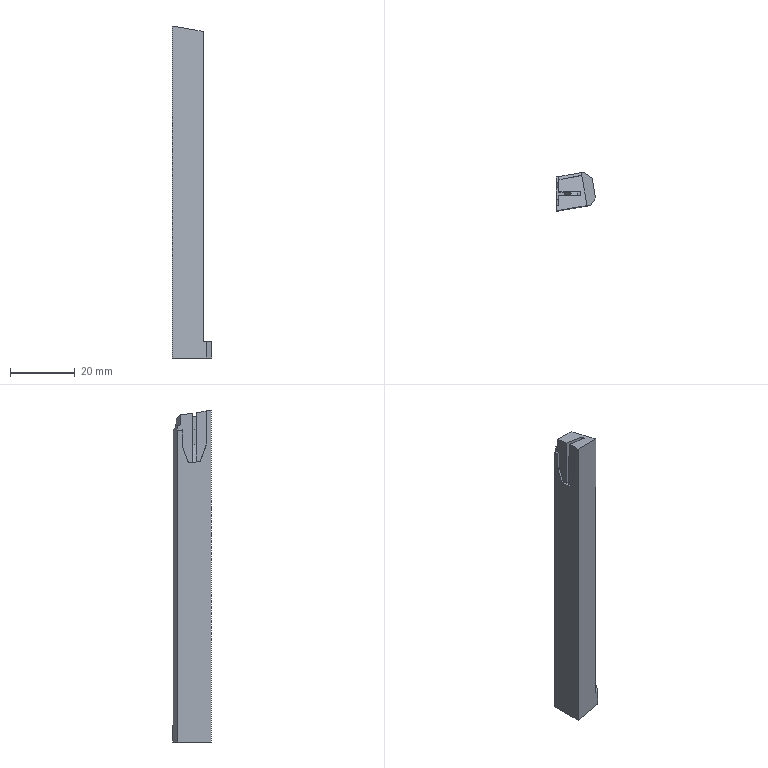Part | STEP file | P011002M003-000 | 1 solid | 27 faces | box 12.084 x 12.031 x 102.825 mm | volume 9089 mm3 | spline 24 | plane 3